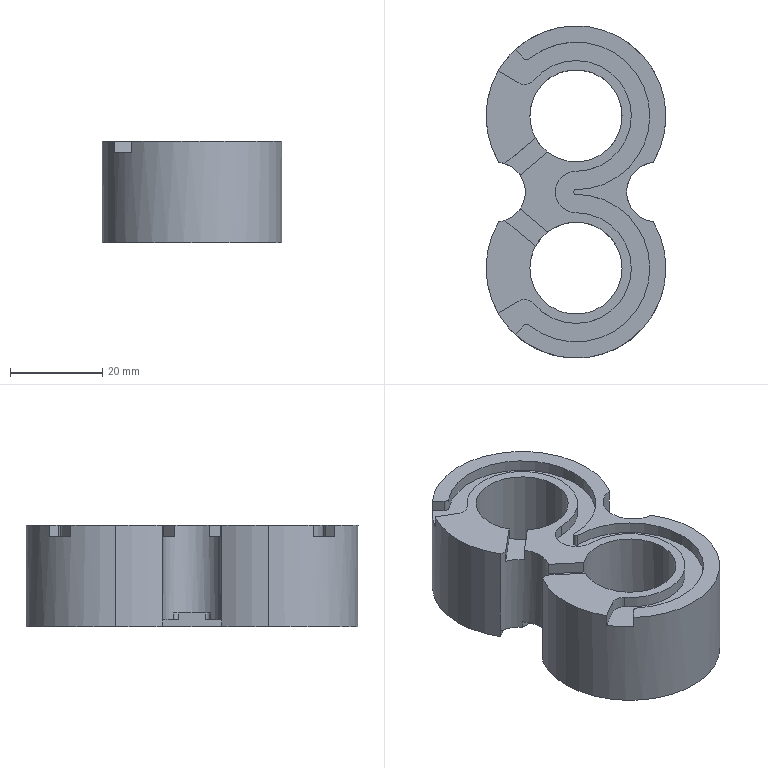Part | SolidWorks | features ICE 5, Fillet 3, Extrusion 1, MirrorPattern 1 | 1 solid | 57 faces | box 39 x 72 x 22 mm | volume 33777 mm3 | cylinder 31 | plane 26 | commonest cylinder face diameters 2 x6 39 x6 20 x4 24 x4 32 x4 13 x3